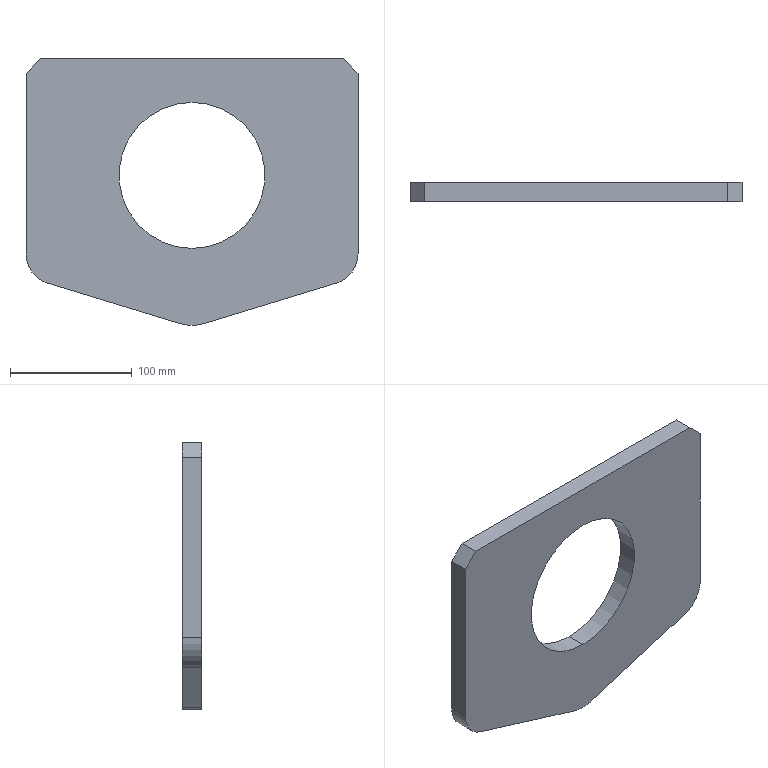Part | SolidWorks | features Extrusion 1 | 1 solid | 15 faces | box 273 x 16 x 219.3 mm | volume 688093 mm3 | plane 9 | cylinder 6 | commonest cylinder face diameters 50 x2 70 x2 120 x2
STEP:
#1=CARTESIAN_POINT('',(0.,16.,-156.));
#2=VERTEX_POINT('',#1);
#3=CARTESIAN_POINT('',(0.,16.,-36.));
#4=VERTEX_POINT('',#3);
#5=CARTESIAN_POINT('',(0.,16.,-96.));
#6=DIRECTION('',(0.,1.,0.));
#7=DIRECTION('',(0.,0.,1.));
#8=AXIS2_PLACEMENT_3D('',#5,#6,#7);
#9=CIRCLE('',#8,60.);
#10=EDGE_CURVE('',#2,#4,#9,.T.);
#11=ORIENTED_EDGE('',*,*,#10,.T.);
#12=CARTESIAN_POINT('',(0.,0.,-36.));
#13=VERTEX_POINT('',#12);
#14=CARTESIAN_POINT('',(0.,16.,-36.));
#15=DIRECTION('',(0.,-1.,0.));
#16=VECTOR('',#15,1000.);
#17=LINE('',#14,#16);
#18=EDGE_CURVE('',#4,#13,#17,.T.);
#19=ORIENTED_EDGE('',*,*,#18,.T.);
#20=CARTESIAN_POINT('',(0.,0.,-156.));
#21=VERTEX_POINT('',#20);
#22=CARTESIAN_POINT('',(0.,0.,-96.));
#23=DIRECTION('',(0.,1.,0.));
#24=DIRECTION('',(0.,0.,1.));
#25=AXIS2_PLACEMENT_3D('',#22,#23,#24);
#26=CIRCLE('',#25,60.);
#27=EDGE_CURVE('',#21,#13,#26,.T.);
#28=ORIENTED_EDGE('',*,*,#27,.F.);
#29=CARTESIAN_POINT('',(0.,16.,-156.));
#30=DIRECTION('',(0.,-1.,0.));
#31=VECTOR('',#30,1000.);
#32=LINE('',#29,#31);
#33=EDGE_CURVE('',#2,#21,#32,.T.);
#34=ORIENTED_EDGE('',*,*,#33,.F.);
#35=EDGE_LOOP('',(#11,#19,#28,#34));
#36=FACE_OUTER_BOUND('',#35,.T.);
#37=CARTESIAN_POINT('',(0.,16.,-96.));
#38=DIRECTION('',(0.,-1.,0.));
#39=DIRECTION('',(0.,0.,-1.));
#40=AXIS2_PLACEMENT_3D('',#37,#38,#39);
#41=CYLINDRICAL_SURFACE('',#40,60.);
#42=ADVANCED_FACE('',(#36),#41,.F.);
#43=CARTESIAN_POINT('',(0.,16.,-219.3));
#44=VERTEX_POINT('',#43);
#45=CARTESIAN_POINT('',(-10.252,16.,-217.765));
#46=VERTEX_POINT('',#45);
#47=CARTESIAN_POINT('',(0.,16.,-184.3));
#48=DIRECTION('',(0.,1.,0.));
#49=DIRECTION('',(0.,0.,1.));
#50=AXIS2_PLACEMENT_3D('',#47,#48,#49);
#51=CIRCLE('',#50,35.);
#52=EDGE_CURVE('',#44,#46,#51,.T.);
#53=ORIENTED_EDGE('',*,*,#52,.F.);
#54=CARTESIAN_POINT('',(0.,0.,-219.3));
#55=VERTEX_POINT('',#54);
#56=CARTESIAN_POINT('',(0.,16.,-219.3));
#57=DIRECTION('',(0.,-1.,0.));
#58=VECTOR('',#57,1000.);
#59=LINE('',#56,#58);
#60=EDGE_CURVE('',#44,#55,#59,.T.);
#61=ORIENTED_EDGE('',*,*,#60,.T.);
#62=CARTESIAN_POINT('',(-10.252,0.,-217.765));
#63=VERTEX_POINT('',#62);
#64=CARTESIAN_POINT('',(0.,0.,-184.3));
#65=DIRECTION('',(0.,1.,0.));
#66=DIRECTION('',(0.,0.,1.));
#67=AXIS2_PLACEMENT_3D('',#64,#65,#66);
#68=CIRCLE('',#67,35.);
#69=EDGE_CURVE('',#55,#63,#68,.T.);
#70=ORIENTED_EDGE('',*,*,#69,.T.);
#71=CARTESIAN_POINT('',(-10.252,16.,-217.765));
#72=DIRECTION('',(0.,-1.,0.));
#73=VECTOR('',#72,1000.);
#74=LINE('',#71,#73);
#75=EDGE_CURVE('',#46,#63,#74,.T.);
#76=ORIENTED_EDGE('',*,*,#75,.F.);
#77=EDGE_LOOP('',(#53,#61,#70,#76));
#78=FACE_OUTER_BOUND('',#77,.T.);
#79=CARTESIAN_POINT('',(0.,16.,-184.3));
#80=DIRECTION('',(0.,-1.,0.));
#81=DIRECTION('',(0.,0.,-1.));
#82=AXIS2_PLACEMENT_3D('',#79,#80,#81);
#83=CYLINDRICAL_SURFACE('',#82,35.);
#84=ADVANCED_FACE('',(#78),#83,.T.);
#85=CARTESIAN_POINT('',(124.5,16.,0.));
#86=VERTEX_POINT('',#85);
#87=CARTESIAN_POINT('',(136.5,16.,-12.));
#88=VERTEX_POINT('',#87);
#89=CARTESIAN_POINT('',(124.5,16.,0.));
#90=DIRECTION('',(0.7071,0.,-0.7071));
#91=VECTOR('',#90,1000.);
#92=LINE('',#89,#91);
#93=EDGE_CURVE('',#86,#88,#92,.T.);
#94=ORIENTED_EDGE('',*,*,#93,.T.);
#95=CARTESIAN_POINT('',(136.5,16.,-160.6));
#96=VERTEX_POINT('',#95);
#97=CARTESIAN_POINT('',(136.5,16.,-12.));
#98=DIRECTION('',(0.,0.,-1.));
#99=VECTOR('',#98,1000.);
#100=LINE('',#97,#99);
#101=EDGE_CURVE('',#88,#96,#100,.T.);
#102=ORIENTED_EDGE('',*,*,#101,.T.);
#103=CARTESIAN_POINT('',(118.823,16.,-184.503));
#104=VERTEX_POINT('',#103);
#105=CARTESIAN_POINT('',(111.5,16.,-160.6));
#106=DIRECTION('',(0.,1.,0.));
#107=DIRECTION('',(0.,0.,1.));
#108=AXIS2_PLACEMENT_3D('',#105,#106,#107);
#109=CIRCLE('',#108,25.);
#110=EDGE_CURVE('',#96,#104,#109,.T.);
#111=ORIENTED_EDGE('',*,*,#110,.T.);
#112=CARTESIAN_POINT('',(10.252,16.,-217.765));
#113=VERTEX_POINT('',#112);
#114=CARTESIAN_POINT('',(10.252,16.,-217.765));
#115=DIRECTION('',(-0.9561,0.,-0.2929));
#116=VECTOR('',#115,1000.);
#117=LINE('',#114,#116);
#118=EDGE_CURVE('',#104,#113,#117,.T.);
#119=ORIENTED_EDGE('',*,*,#118,.T.);
#120=CARTESIAN_POINT('',(0.,16.,-184.3));
#121=DIRECTION('',(0.,1.,0.));
#122=DIRECTION('',(0.,0.,1.));
#123=AXIS2_PLACEMENT_3D('',#120,#121,#122);
#124=CIRCLE('',#123,35.);
#125=EDGE_CURVE('',#113,#44,#124,.T.);
#126=ORIENTED_EDGE('',*,*,#125,.T.);
#127=ORIENTED_EDGE('',*,*,#52,.T.);
#128=CARTESIAN_POINT('',(-118.823,16.,-184.503));
#129=VERTEX_POINT('',#128);
#130=CARTESIAN_POINT('',(-10.252,16.,-217.765));
#131=DIRECTION('',(-0.9561,0.,0.2929));
#132=VECTOR('',#131,1000.);
#133=LINE('',#130,#132);
#134=EDGE_CURVE('',#46,#129,#133,.T.);
#135=ORIENTED_EDGE('',*,*,#134,.T.);
#136=CARTESIAN_POINT('',(-136.5,16.,-160.6));
#137=VERTEX_POINT('',#136);
#138=CARTESIAN_POINT('',(-111.5,16.,-160.6));
#139=DIRECTION('',(0.,1.,0.));
#140=DIRECTION('',(0.,0.,-1.));
#141=AXIS2_PLACEMENT_3D('',#138,#139,#140);
#142=CIRCLE('',#141,25.);
#143=EDGE_CURVE('',#129,#137,#142,.T.);
#144=ORIENTED_EDGE('',*,*,#143,.T.);
#145=CARTESIAN_POINT('',(-136.5,16.,-12.));
#146=VERTEX_POINT('',#145);
#147=CARTESIAN_POINT('',(-136.5,16.,-12.));
#148=DIRECTION('',(0.,0.,1.));
#149=VECTOR('',#148,1000.);
#150=LINE('',#147,#149);
#151=EDGE_CURVE('',#137,#146,#150,.T.);
#152=ORIENTED_EDGE('',*,*,#151,.T.);
#153=CARTESIAN_POINT('',(-124.5,16.,0.));
#154=VERTEX_POINT('',#153);
#155=CARTESIAN_POINT('',(-124.5,16.,0.));
#156=DIRECTION('',(0.7071,0.,0.7071));
#157=VECTOR('',#156,1000.);
#158=LINE('',#155,#157);
#159=EDGE_CURVE('',#146,#154,#158,.T.);
#160=ORIENTED_EDGE('',*,*,#159,.T.);
#161=CARTESIAN_POINT('',(-124.5,16.,0.));
#162=DIRECTION('',(1.,0.,0.));
#163=VECTOR('',#162,1000.);
#164=LINE('',#161,#163);
#165=EDGE_CURVE('',#154,#86,#164,.T.);
#166=ORIENTED_EDGE('',*,*,#165,.T.);
#167=EDGE_LOOP('',(#94,#102,#111,#119,#126,#127,#135,#144,#152,#160,#166));
#168=FACE_OUTER_BOUND('',#167,.T.);
#169=ORIENTED_EDGE('',*,*,#10,.F.);
#170=CARTESIAN_POINT('',(0.,16.,-96.));
#171=DIRECTION('',(0.,1.,0.));
#172=DIRECTION('',(0.,0.,1.));
#173=AXIS2_PLACEMENT_3D('',#170,#171,#172);
#174=CIRCLE('',#173,60.);
#175=EDGE_CURVE('',#4,#2,#174,.T.);
#176=ORIENTED_EDGE('',*,*,#175,.F.);
#177=EDGE_LOOP('',(#169,#176));
#178=FACE_BOUND('',#177,.T.);
#179=CARTESIAN_POINT('',(111.5,16.,-160.6));
#180=DIRECTION('',(0.,1.,0.));
#181=DIRECTION('',(0.,0.,1.));
#182=AXIS2_PLACEMENT_3D('',#179,#180,#181);
#183=PLANE('',#182);
#184=ADVANCED_FACE('',(#168,#178),#183,.T.);
#185=CARTESIAN_POINT('',(124.5,0.,0.));
#186=VERTEX_POINT('',#185);
#187=CARTESIAN_POINT('',(136.5,0.,-12.));
#188=VERTEX_POINT('',#187);
#189=CARTESIAN_POINT('',(124.5,0.,0.));
#190=DIRECTION('',(0.7071,0.,-0.7071));
#191=VECTOR('',#190,1000.);
#192=LINE('',#189,#191);
#193=EDGE_CURVE('',#186,#188,#192,.T.);
#194=ORIENTED_EDGE('',*,*,#193,.F.);
#195=CARTESIAN_POINT('',(-124.5,0.,0.));
#196=VERTEX_POINT('',#195);
#197=CARTESIAN_POINT('',(-124.5,0.,0.));
#198=DIRECTION('',(1.,0.,0.));
#199=VECTOR('',#198,1000.);
#200=LINE('',#197,#199);
#201=EDGE_CURVE('',#196,#186,#200,.T.);
#202=ORIENTED_EDGE('',*,*,#201,.F.);
#203=CARTESIAN_POINT('',(-136.5,0.,-12.));
#204=VERTEX_POINT('',#203);
#205=CARTESIAN_POINT('',(-124.5,0.,0.));
#206=DIRECTION('',(0.7071,0.,0.7071));
#207=VECTOR('',#206,1000.);
#208=LINE('',#205,#207);
#209=EDGE_CURVE('',#204,#196,#208,.T.);
#210=ORIENTED_EDGE('',*,*,#209,.F.);
#211=CARTESIAN_POINT('',(-136.5,0.,-160.6));
#212=VERTEX_POINT('',#211);
#213=CARTESIAN_POINT('',(-136.5,0.,-12.));
#214=DIRECTION('',(0.,0.,1.));
#215=VECTOR('',#214,1000.);
#216=LINE('',#213,#215);
#217=EDGE_CURVE('',#212,#204,#216,.T.);
#218=ORIENTED_EDGE('',*,*,#217,.F.);
#219=CARTESIAN_POINT('',(-118.823,0.,-184.503));
#220=VERTEX_POINT('',#219);
#221=CARTESIAN_POINT('',(-111.5,0.,-160.6));
#222=DIRECTION('',(0.,1.,0.));
#223=DIRECTION('',(0.,0.,-1.));
#224=AXIS2_PLACEMENT_3D('',#221,#222,#223);
#225=CIRCLE('',#224,25.);
#226=EDGE_CURVE('',#220,#212,#225,.T.);
#227=ORIENTED_EDGE('',*,*,#226,.F.);
#228=CARTESIAN_POINT('',(-10.252,0.,-217.765));
#229=DIRECTION('',(-0.9561,0.,0.2929));
#230=VECTOR('',#229,1000.);
#231=LINE('',#228,#230);
#232=EDGE_CURVE('',#63,#220,#231,.T.);
#233=ORIENTED_EDGE('',*,*,#232,.F.);
#234=ORIENTED_EDGE('',*,*,#69,.F.);
#235=CARTESIAN_POINT('',(10.252,0.,-217.765));
#236=VERTEX_POINT('',#235);
#237=CARTESIAN_POINT('',(0.,0.,-184.3));
#238=DIRECTION('',(0.,1.,0.));
#239=DIRECTION('',(0.,0.,1.));
#240=AXIS2_PLACEMENT_3D('',#237,#238,#239);
#241=CIRCLE('',#240,35.);
#242=EDGE_CURVE('',#236,#55,#241,.T.);
#243=ORIENTED_EDGE('',*,*,#242,.F.);
#244=CARTESIAN_POINT('',(118.823,0.,-184.503));
#245=VERTEX_POINT('',#244);
#246=CARTESIAN_POINT('',(10.252,0.,-217.765));
#247=DIRECTION('',(-0.9561,0.,-0.2929));
#248=VECTOR('',#247,1000.);
#249=LINE('',#246,#248);
#250=EDGE_CURVE('',#245,#236,#249,.T.);
#251=ORIENTED_EDGE('',*,*,#250,.F.);
#252=CARTESIAN_POINT('',(136.5,0.,-160.6));
#253=VERTEX_POINT('',#252);
#254=CARTESIAN_POINT('',(111.5,0.,-160.6));
#255=DIRECTION('',(0.,1.,0.));
#256=DIRECTION('',(0.,0.,1.));
#257=AXIS2_PLACEMENT_3D('',#254,#255,#256);
#258=CIRCLE('',#257,25.);
#259=EDGE_CURVE('',#253,#245,#258,.T.);
#260=ORIENTED_EDGE('',*,*,#259,.F.);
#261=CARTESIAN_POINT('',(136.5,0.,-12.));
#262=DIRECTION('',(0.,0.,-1.));
#263=VECTOR('',#262,1000.);
#264=LINE('',#261,#263);
#265=EDGE_CURVE('',#188,#253,#264,.T.);
#266=ORIENTED_EDGE('',*,*,#265,.F.);
#267=EDGE_LOOP('',(#194,#202,#210,#218,#227,#233,#234,#243,#251,#260,#266));
#268=FACE_OUTER_BOUND('',#267,.T.);
#269=ORIENTED_EDGE('',*,*,#27,.T.);
#270=CARTESIAN_POINT('',(0.,0.,-96.));
#271=DIRECTION('',(0.,1.,0.));
#272=DIRECTION('',(0.,0.,1.));
#273=AXIS2_PLACEMENT_3D('',#270,#271,#272);
#274=CIRCLE('',#273,60.);
#275=EDGE_CURVE('',#13,#21,#274,.T.);
#276=ORIENTED_EDGE('',*,*,#275,.T.);
#277=EDGE_LOOP('',(#269,#276));
#278=FACE_BOUND('',#277,.T.);
#279=CARTESIAN_POINT('',(111.5,0.,-160.6));
#280=DIRECTION('',(0.,1.,0.));
#281=DIRECTION('',(0.,0.,1.));
#282=AXIS2_PLACEMENT_3D('',#279,#280,#281);
#283=PLANE('',#282);
#284=ADVANCED_FACE('',(#268,#278),#283,.F.);
#285=ORIENTED_EDGE('',*,*,#193,.T.);
#286=CARTESIAN_POINT('',(136.5,16.,-12.));
#287=DIRECTION('',(0.,-1.,0.));
#288=VECTOR('',#287,1000.);
#289=LINE('',#286,#288);
#290=EDGE_CURVE('',#88,#188,#289,.T.);
#291=ORIENTED_EDGE('',*,*,#290,.F.);
#292=ORIENTED_EDGE('',*,*,#93,.F.);
#293=CARTESIAN_POINT('',(124.5,16.,0.));
#294=DIRECTION('',(0.,-1.,0.));
#295=VECTOR('',#294,1000.);
#296=LINE('',#293,#295);
#297=EDGE_CURVE('',#86,#186,#296,.T.);
#298=ORIENTED_EDGE('',*,*,#297,.T.);
#299=EDGE_LOOP('',(#285,#291,#292,#298));
#300=FACE_OUTER_BOUND('',#299,.T.);
#301=CARTESIAN_POINT('',(124.5,16.,0.));
#302=DIRECTION('',(-0.7071,0.,-0.7071));
#303=DIRECTION('',(-0.7071,0.,0.7071));
#304=AXIS2_PLACEMENT_3D('',#301,#302,#303);
#305=PLANE('',#304);
#306=ADVANCED_FACE('',(#300),#305,.F.);
#307=ORIENTED_EDGE('',*,*,#265,.T.);
#308=CARTESIAN_POINT('',(136.5,16.,-160.6));
#309=DIRECTION('',(0.,-1.,0.));
#310=VECTOR('',#309,1000.);
#311=LINE('',#308,#310);
#312=EDGE_CURVE('',#96,#253,#311,.T.);
#313=ORIENTED_EDGE('',*,*,#312,.F.);
#314=ORIENTED_EDGE('',*,*,#101,.F.);
#315=ORIENTED_EDGE('',*,*,#290,.T.);
#316=EDGE_LOOP('',(#307,#313,#314,#315));
#317=FACE_OUTER_BOUND('',#316,.T.);
#318=CARTESIAN_POINT('',(136.5,16.,-12.));
#319=DIRECTION('',(-1.,0.,0.));
#320=DIRECTION('',(0.,0.,1.));
#321=AXIS2_PLACEMENT_3D('',#318,#319,#320);
#322=PLANE('',#321);
#323=ADVANCED_FACE('',(#317),#322,.F.);
#324=ORIENTED_EDGE('',*,*,#259,.T.);
#325=CARTESIAN_POINT('',(118.823,16.,-184.503));
#326=DIRECTION('',(0.,-1.,0.));
#327=VECTOR('',#326,1000.);
#328=LINE('',#325,#327);
#329=EDGE_CURVE('',#104,#245,#328,.T.);
#330=ORIENTED_EDGE('',*,*,#329,.F.);
#331=ORIENTED_EDGE('',*,*,#110,.F.);
#332=ORIENTED_EDGE('',*,*,#312,.T.);
#333=EDGE_LOOP('',(#324,#330,#331,#332));
#334=FACE_OUTER_BOUND('',#333,.T.);
#335=CARTESIAN_POINT('',(111.5,16.,-160.6));
#336=DIRECTION('',(0.,-1.,0.));
#337=DIRECTION('',(0.,0.,-1.));
#338=AXIS2_PLACEMENT_3D('',#335,#336,#337);
#339=CYLINDRICAL_SURFACE('',#338,25.);
#340=ADVANCED_FACE('',(#334),#339,.T.);
#341=ORIENTED_EDGE('',*,*,#250,.T.);
#342=CARTESIAN_POINT('',(10.252,16.,-217.765));
#343=DIRECTION('',(0.,-1.,0.));
#344=VECTOR('',#343,1000.);
#345=LINE('',#342,#344);
#346=EDGE_CURVE('',#113,#236,#345,.T.);
#347=ORIENTED_EDGE('',*,*,#346,.F.);
#348=ORIENTED_EDGE('',*,*,#118,.F.);
#349=ORIENTED_EDGE('',*,*,#329,.T.);
#350=EDGE_LOOP('',(#341,#347,#348,#349));
#351=FACE_OUTER_BOUND('',#350,.T.);
#352=CARTESIAN_POINT('',(10.252,16.,-217.765));
#353=DIRECTION('',(-0.2929,0.,0.9561));
#354=DIRECTION('',(0.9561,0.,0.2929));
#355=AXIS2_PLACEMENT_3D('',#352,#353,#354);
#356=PLANE('',#355);
#357=ADVANCED_FACE('',(#351),#356,.F.);
#358=ORIENTED_EDGE('',*,*,#60,.F.);
#359=ORIENTED_EDGE('',*,*,#125,.F.);
#360=ORIENTED_EDGE('',*,*,#346,.T.);
#361=ORIENTED_EDGE('',*,*,#242,.T.);
#362=EDGE_LOOP('',(#358,#359,#360,#361));
#363=FACE_OUTER_BOUND('',#362,.T.);
#364=CARTESIAN_POINT('',(0.,16.,-184.3));
#365=DIRECTION('',(0.,-1.,0.));
#366=DIRECTION('',(0.,0.,-1.));
#367=AXIS2_PLACEMENT_3D('',#364,#365,#366);
#368=CYLINDRICAL_SURFACE('',#367,35.);
#369=ADVANCED_FACE('',(#363),#368,.T.);
#370=ORIENTED_EDGE('',*,*,#232,.T.);
#371=CARTESIAN_POINT('',(-118.823,16.,-184.503));
#372=DIRECTION('',(0.,-1.,0.));
#373=VECTOR('',#372,1000.);
#374=LINE('',#371,#373);
#375=EDGE_CURVE('',#129,#220,#374,.T.);
#376=ORIENTED_EDGE('',*,*,#375,.F.);
#377=ORIENTED_EDGE('',*,*,#134,.F.);
#378=ORIENTED_EDGE('',*,*,#75,.T.);
#379=EDGE_LOOP('',(#370,#376,#377,#378));
#380=FACE_OUTER_BOUND('',#379,.T.);
#381=CARTESIAN_POINT('',(-10.252,16.,-217.765));
#382=DIRECTION('',(0.2929,0.,0.9561));
#383=DIRECTION('',(0.9561,0.,-0.2929));
#384=AXIS2_PLACEMENT_3D('',#381,#382,#383);
#385=PLANE('',#384);
#386=ADVANCED_FACE('',(#380),#385,.F.);
#387=ORIENTED_EDGE('',*,*,#226,.T.);
#388=CARTESIAN_POINT('',(-136.5,16.,-160.6));
#389=DIRECTION('',(0.,-1.,0.));
#390=VECTOR('',#389,1000.);
#391=LINE('',#388,#390);
#392=EDGE_CURVE('',#137,#212,#391,.T.);
#393=ORIENTED_EDGE('',*,*,#392,.F.);
#394=ORIENTED_EDGE('',*,*,#143,.F.);
#395=ORIENTED_EDGE('',*,*,#375,.T.);
#396=EDGE_LOOP('',(#387,#393,#394,#395));
#397=FACE_OUTER_BOUND('',#396,.T.);
#398=CARTESIAN_POINT('',(-111.5,16.,-160.6));
#399=DIRECTION('',(0.,-1.,0.));
#400=DIRECTION('',(0.,0.,-1.));
#401=AXIS2_PLACEMENT_3D('',#398,#399,#400);
#402=CYLINDRICAL_SURFACE('',#401,25.);
#403=ADVANCED_FACE('',(#397),#402,.T.);
#404=ORIENTED_EDGE('',*,*,#217,.T.);
#405=CARTESIAN_POINT('',(-136.5,16.,-12.));
#406=DIRECTION('',(0.,-1.,0.));
#407=VECTOR('',#406,1000.);
#408=LINE('',#405,#407);
#409=EDGE_CURVE('',#146,#204,#408,.T.);
#410=ORIENTED_EDGE('',*,*,#409,.F.);
#411=ORIENTED_EDGE('',*,*,#151,.F.);
#412=ORIENTED_EDGE('',*,*,#392,.T.);
#413=EDGE_LOOP('',(#404,#410,#411,#412));
#414=FACE_OUTER_BOUND('',#413,.T.);
#415=CARTESIAN_POINT('',(-136.5,16.,-12.));
#416=DIRECTION('',(1.,0.,0.));
#417=DIRECTION('',(0.,0.,-1.));
#418=AXIS2_PLACEMENT_3D('',#415,#416,#417);
#419=PLANE('',#418);
#420=ADVANCED_FACE('',(#414),#419,.F.);
#421=ORIENTED_EDGE('',*,*,#209,.T.);
#422=CARTESIAN_POINT('',(-124.5,16.,0.));
#423=DIRECTION('',(0.,-1.,0.));
#424=VECTOR('',#423,1000.);
#425=LINE('',#422,#424);
#426=EDGE_CURVE('',#154,#196,#425,.T.);
#427=ORIENTED_EDGE('',*,*,#426,.F.);
#428=ORIENTED_EDGE('',*,*,#159,.F.);
#429=ORIENTED_EDGE('',*,*,#409,.T.);
#430=EDGE_LOOP('',(#421,#427,#428,#429));
#431=FACE_OUTER_BOUND('',#430,.T.);
#432=CARTESIAN_POINT('',(-124.5,16.,0.));
#433=DIRECTION('',(0.7071,0.,-0.7071));
#434=DIRECTION('',(-0.7071,0.,-0.7071));
#435=AXIS2_PLACEMENT_3D('',#432,#433,#434);
#436=PLANE('',#435);
#437=ADVANCED_FACE('',(#431),#436,.F.);
#438=ORIENTED_EDGE('',*,*,#201,.T.);
#439=ORIENTED_EDGE('',*,*,#297,.F.);
#440=ORIENTED_EDGE('',*,*,#165,.F.);
#441=ORIENTED_EDGE('',*,*,#426,.T.);
#442=EDGE_LOOP('',(#438,#439,#440,#441));
#443=FACE_OUTER_BOUND('',#442,.T.);
#444=CARTESIAN_POINT('',(-124.5,16.,0.));
#445=DIRECTION('',(0.,0.,-1.));
#446=DIRECTION('',(-1.,0.,0.));
#447=AXIS2_PLACEMENT_3D('',#444,#445,#446);
#448=PLANE('',#447);
#449=ADVANCED_FACE('',(#443),#448,.F.);
#450=ORIENTED_EDGE('',*,*,#18,.F.);
#451=ORIENTED_EDGE('',*,*,#175,.T.);
#452=ORIENTED_EDGE('',*,*,#33,.T.);
#453=ORIENTED_EDGE('',*,*,#275,.F.);
#454=EDGE_LOOP('',(#450,#451,#452,#453));
#455=FACE_OUTER_BOUND('',#454,.T.);
#456=CARTESIAN_POINT('',(0.,16.,-96.));
#457=DIRECTION('',(0.,-1.,0.));
#458=DIRECTION('',(0.,0.,-1.));
#459=AXIS2_PLACEMENT_3D('',#456,#457,#458);
#460=CYLINDRICAL_SURFACE('',#459,60.);
#461=ADVANCED_FACE('',(#455),#460,.F.);
#462=CLOSED_SHELL('',(#42,#84,#184,#284,#306,#323,#340,#357,#369,#386,#403,#420,#437,#449,#461));
#463=MANIFOLD_SOLID_BREP('',#462);
#464=CARTESIAN_POINT('',(0.,0.,0.));
#465=DIRECTION('',(0.,0.,1.));
#466=DIRECTION('',(1.,0.,0.));
#467=AXIS2_PLACEMENT_3D('',#464,#465,#466);
#468=(LENGTH_UNIT()NAMED_UNIT(*)SI_UNIT(.MILLI.,.METRE.));
#469=UNCERTAINTY_MEASURE_WITH_UNIT(LENGTH_MEASURE(0.00001),#468,'','');
#470=(NAMED_UNIT(*)PLANE_ANGLE_UNIT()SI_UNIT($,.RADIAN.));
#471=(NAMED_UNIT(*)SI_UNIT($,.STERADIAN.)SOLID_ANGLE_UNIT());
#472=(GEOMETRIC_REPRESENTATION_CONTEXT(3)GLOBAL_UNCERTAINTY_ASSIGNED_CONTEXT((#469))GLOBAL_UNIT_ASSIGNED_CONTEXT((#468,#470,#471))REPRESENTATION_CONTEXT('',''));
#473=ADVANCED_BREP_SHAPE_REPRESENTATION('',(#463,#467),#472);